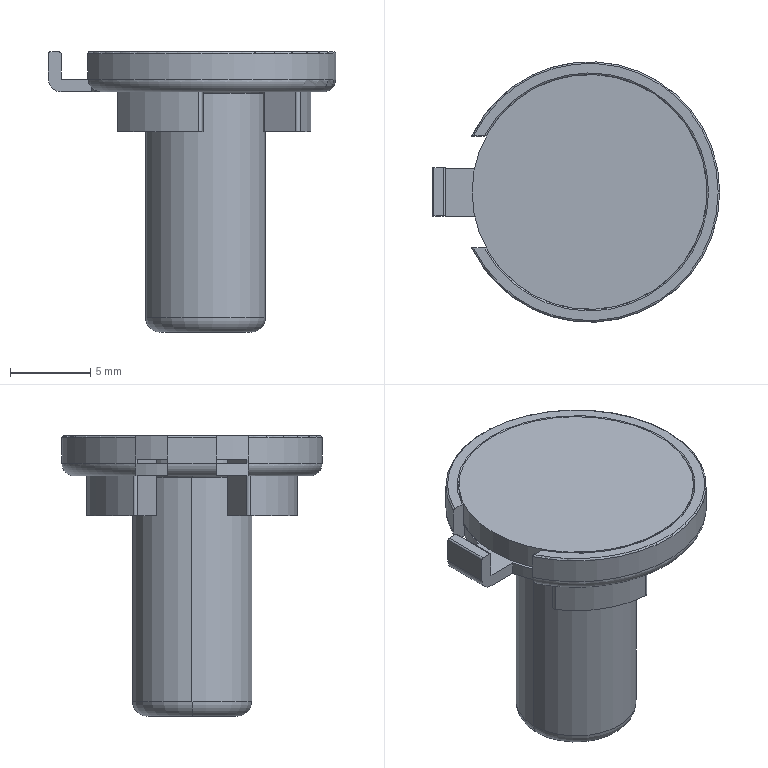NC program | NX | posted with a generic post | part box 17.958 x 16.273 x 17.5 mm
Lines 4450 to 5539 of 11029:
(ZLEVEL_PROFILE_COPY_COPY_2_COPY_1_COPY , TOOL : D1)
N8886 T12 M6
N8888 G54
N8890 G17 G0 G90 X-0.541 Y-4.574 S8005 M3
N8892 G43 Z30. H12
N8894 Z-0.08
N8896 G94 G1 X-0.394 Y-4.482 F850.
N8898 X-0.36 Y-4.465
N8900 X-0.342 Y-4.431
N8902 X-0.347 Y-4.394
N8904 X-0.353 Y-4.21
N8906 G2 X0.289 Y-3.488 R0.7
N8908 G3 X2.876 Y-1.994 R3.5
N8910 G2 X3.823 Y-1.799 R0.7
N8912 G1 X3.978 Y-1.896
N8914 X4.008 Y-1.919
N8916 X4.047 Y-1.92
N8918 X4.078 Y-1.9
N8920 X4.231 Y-1.819
N8922 G0 Z30.
N8924 Y1.819
N8926 Z-0.08
N8928 G1 X4.078 Y1.9
N8930 X4.047 Y1.92
N8932 X4.008 Y1.919
N8934 X3.978 Y1.896
N8936 X3.823 Y1.799
N8938 G2 X2.876 Y1.994 R0.7
N8940 G3 X0.289 Y3.488 R3.5
N8942 G2 X-0.353 Y4.21 R0.7
N8944 G1 X-0.347 Y4.394
N8946 X-0.342 Y4.431
N8948 X-0.36 Y4.465
N8950 X-0.394 Y4.482
N8952 X-0.541 Y4.574
N8954 G0 Z30.
N8956 X-3.69 Y2.755
N8958 Z-0.08
N8960 G1 X-3.684 Y2.582
N8962 X-3.687 Y2.544
N8964 X-3.666 Y2.512
N8966 X-3.631 Y2.497
N8968 X-3.469 Y2.411
N8970 G2 X-3.165 Y1.494 R0.7
N8972 G3 X-3.165 Y-1.494 R3.5
N8974 G2 X-3.469 Y-2.411 R0.7
N8976 G1 X-3.631 Y-2.497
N8978 X-3.666 Y-2.512
N8980 X-3.687 Y-2.544
N8982 X-3.684 Y-2.582
N8984 X-3.69 Y-2.755
N8986 G0 Z30.
N8988 X-2.316 Y-2.821
N8990 Z-0.08
N8992 G1 X-2.281 Y-2.656
N8994 X-2.27 Y-2.62
N8996 X-2.281 Y-2.584
N8998 X-2.312 Y-2.561
N9000 G2 X-2.312 Y2.561 R3.45
N9002 G1 X-2.281 Y2.584
N9004 X-2.27 Y2.62
N9006 X-2.281 Y2.656
N9008 X-2.316 Y2.821
N9010 G0 Z30.
N9012 Y-2.821
N9014 Z-0.159
N9016 G1 X-2.281 Y-2.656
N9018 X-2.27 Y-2.62
N9020 X-2.281 Y-2.584
N9022 X-2.312 Y-2.561
N9024 G2 X-2.312 Y2.561 R3.45
N9026 G1 X-2.281 Y2.584
N9028 X-2.27 Y2.62
N9030 X-2.281 Y2.656
N9032 X-2.316 Y2.821
N9034 G0 Z30.
N9036 X-3.69 Y2.755
N9038 Z-0.159
N9040 G1 X-3.684 Y2.582
N9042 X-3.687 Y2.544
N9044 X-3.666 Y2.512
N9046 X-3.631 Y2.497
N9048 X-3.469 Y2.411
N9050 G2 X-3.165 Y1.494 R0.7
N9052 G3 X-3.165 Y-1.494 R3.5
N9054 G2 X-3.469 Y-2.411 R0.7
N9056 G1 X-3.631 Y-2.497
N9058 X-3.666 Y-2.512
N9060 X-3.687 Y-2.544
N9062 X-3.684 Y-2.582
N9064 X-3.69 Y-2.755
N9066 G0 Z30.
N9068 Y2.755
N9070 Z-0.239
N9072 G1 X-3.684 Y2.582
N9074 X-3.687 Y2.544
N9076 X-3.666 Y2.512
N9078 X-3.631 Y2.497
N9080 X-3.469 Y2.411
N9082 G2 X-3.165 Y1.494 R0.7
N9084 G3 X-3.165 Y-1.494 R3.5
N9086 G2 X-3.469 Y-2.411 R0.7
N9088 G1 X-3.631 Y-2.497
N9090 X-3.666 Y-2.512
N9092 X-3.687 Y-2.544
N9094 X-3.684 Y-2.582
N9096 X-3.69 Y-2.755
N9098 G0 Z30.
N9100 X-2.316 Y-2.821
N9102 Z-0.239
N9104 G1 X-2.281 Y-2.656
N9106 X-2.27 Y-2.62
N9108 X-2.281 Y-2.584
N9110 X-2.312 Y-2.561
N9112 G2 X-2.312 Y2.561 R3.45
N9114 G1 X-2.281 Y2.584
N9116 X-2.27 Y2.62
N9118 X-2.281 Y2.656
N9120 X-2.316 Y2.821
N9122 G0 Z30.
N9124 Y-2.821
N9126 Z-0.318
N9128 G1 X-2.281 Y-2.656
N9130 X-2.27 Y-2.62
N9132 X-2.281 Y-2.584
N9134 X-2.312 Y-2.561
N9136 G2 X-2.312 Y2.561 R3.45
N9138 G1 X-2.281 Y2.584
N9140 X-2.27 Y2.62
N9142 X-2.281 Y2.656
N9144 X-2.316 Y2.821
N9146 G0 Z30.
N9148 X-3.69 Y2.755
N9150 Z-0.318
N9152 G1 X-3.684 Y2.582
N9154 X-3.687 Y2.544
N9156 X-3.666 Y2.512
N9158 X-3.631 Y2.497
N9160 X-3.469 Y2.411
N9162 G2 X-3.165 Y1.494 R0.7
N9164 G3 X-3.165 Y-1.494 R3.5
N9166 G2 X-3.469 Y-2.411 R0.7
N9168 G1 X-3.631 Y-2.497
N9170 X-3.666 Y-2.512
N9172 X-3.687 Y-2.544
N9174 X-3.684 Y-2.582
N9176 X-3.69 Y-2.755
N9178 G0 Z30.
N9180 Y2.755
N9182 Z-0.398
N9184 G1 X-3.684 Y2.582
N9186 X-3.687 Y2.544
N9188 X-3.666 Y2.512
N9190 X-3.631 Y2.497
N9192 X-3.469 Y2.411
N9194 G2 X-3.165 Y1.494 R0.7
N9196 G3 X-3.165 Y-1.494 R3.5
N9198 G2 X-3.469 Y-2.411 R0.7
N9200 G1 X-3.631 Y-2.497
N9202 X-3.666 Y-2.512
N9204 X-3.687 Y-2.544
N9206 X-3.684 Y-2.582
N9208 X-3.69 Y-2.755
N9210 G0 Z30.
N9212 X-2.316 Y-2.821
N9214 Z-0.398
N9216 G1 X-2.281 Y-2.656
N9218 X-2.27 Y-2.62
N9220 X-2.281 Y-2.584
N9222 X-2.312 Y-2.561
N9224 G2 X-2.312 Y2.561 R3.45
N9226 G1 X-2.281 Y2.584
N9228 X-2.27 Y2.62
N9230 X-2.281 Y2.656
N9232 X-2.316 Y2.821
N9234 G0 Z30.
N9236 Y-2.821
N9238 Z-0.477
N9240 G1 X-2.281 Y-2.656
N9242 X-2.27 Y-2.62
N9244 X-2.281 Y-2.584
N9246 X-2.312 Y-2.561
N9248 G2 X-2.312 Y2.561 R3.45
N9250 G1 X-2.281 Y2.584
N9252 X-2.27 Y2.62
N9254 X-2.281 Y2.656
N9256 X-2.316 Y2.821
N9258 G0 Z30.
N9260 X-3.69 Y2.755
N9262 Z-0.477
N9264 G1 X-3.684 Y2.582
N9266 X-3.687 Y2.544
N9268 X-3.666 Y2.512
N9270 X-3.631 Y2.497
N9272 X-3.469 Y2.411
N9274 G2 X-3.165 Y1.494 R0.7
N9276 G3 X-3.165 Y-1.494 R3.5
N9278 G2 X-3.469 Y-2.411 R0.7
N9280 G1 X-3.631 Y-2.497
N9282 X-3.666 Y-2.512
N9284 X-3.687 Y-2.544
N9286 X-3.684 Y-2.582
N9288 X-3.69 Y-2.755
N9290 G0 Z30.
N9292 Y2.755
N9294 Z-0.557
N9296 G1 X-3.684 Y2.582
N9298 X-3.687 Y2.544
N9300 X-3.666 Y2.512
N9302 X-3.631 Y2.497
N9304 X-3.469 Y2.411
N9306 G2 X-3.165 Y1.494 R0.7
N9308 G3 X-3.165 Y-1.494 R3.5
N9310 G2 X-3.469 Y-2.411 R0.7
N9312 G1 X-3.631 Y-2.497
N9314 X-3.666 Y-2.512
N9316 X-3.687 Y-2.544
N9318 X-3.684 Y-2.582
N9320 X-3.69 Y-2.755
N9322 G0 Z30.
N9324 X-2.316 Y-2.821
N9326 Z-0.557
N9328 G1 X-2.281 Y-2.656
N9330 X-2.27 Y-2.62
N9332 X-2.281 Y-2.584
N9334 X-2.312 Y-2.561
N9336 G2 X-2.312 Y2.561 R3.45
N9338 G1 X-2.281 Y2.584
N9340 X-2.27 Y2.62
N9342 X-2.281 Y2.656
N9344 X-2.316 Y2.821
N9346 G0 Z30.
N9348 Y-2.821
N9350 Z-0.636
N9352 G1 X-2.281 Y-2.656
N9354 X-2.27 Y-2.62
N9356 X-2.281 Y-2.584
N9358 X-2.312 Y-2.561
N9360 G2 X-2.312 Y2.561 R3.45
N9362 G1 X-2.281 Y2.584
N9364 X-2.27 Y2.62
N9366 X-2.281 Y2.656
N9368 X-2.316 Y2.821
N9370 G0 Z30.
N9372 X-3.69 Y2.755
N9374 Z-0.636
N9376 G1 X-3.684 Y2.582
N9378 X-3.687 Y2.544
N9380 X-3.666 Y2.512
N9382 X-3.631 Y2.497
N9384 X-3.469 Y2.411
N9386 G2 X-3.165 Y1.494 R0.7
N9388 G3 X-3.165 Y-1.494 R3.5
N9390 G2 X-3.469 Y-2.411 R0.7
N9392 G1 X-3.631 Y-2.497
N9394 X-3.666 Y-2.512
N9396 X-3.687 Y-2.544
N9398 X-3.684 Y-2.582
N9400 X-3.69 Y-2.755
N9402 G0 Z30.
N9404 Y2.755
N9406 Z-0.716
N9408 G1 X-3.684 Y2.582
N9410 X-3.687 Y2.544
N9412 X-3.666 Y2.512
N9414 X-3.631 Y2.497
N9416 X-3.469 Y2.411
N9418 G2 X-3.165 Y1.494 R0.7
N9420 G3 X-3.165 Y-1.494 R3.5
N9422 G2 X-3.469 Y-2.411 R0.7
N9424 G1 X-3.631 Y-2.497
N9426 X-3.666 Y-2.512
N9428 X-3.687 Y-2.544
N9430 X-3.684 Y-2.582
N9432 X-3.69 Y-2.755
N9434 G0 Z30.
N9436 X-2.316 Y-2.821
N9438 Z-0.716
N9440 G1 X-2.281 Y-2.656
N9442 X-2.27 Y-2.62
N9444 X-2.281 Y-2.584
N9446 X-2.312 Y-2.561
N9448 G2 X-2.312 Y2.561 R3.45
N9450 G1 X-2.281 Y2.584
N9452 X-2.27 Y2.62
N9454 X-2.281 Y2.656
N9456 X-2.316 Y2.821
N9458 G0 Z30.
N9460 Y-2.821
N9462 Z-0.795
N9464 G1 X-2.281 Y-2.656
N9466 X-2.27 Y-2.62
N9468 X-2.281 Y-2.584
N9470 X-2.312 Y-2.561
N9472 G2 X-2.312 Y2.561 R3.45
N9474 G1 X-2.281 Y2.584
N9476 X-2.27 Y2.62
N9478 X-2.281 Y2.656
N9480 X-2.316 Y2.821
N9482 G0 Z30.
N9484 X-3.69 Y2.755
N9486 Z-0.795
N9488 G1 X-3.684 Y2.582
N9490 X-3.687 Y2.544
N9492 X-3.666 Y2.512
N9494 X-3.631 Y2.497
N9496 X-3.469 Y2.411
N9498 G2 X-3.165 Y1.494 R0.7
N9500 G3 X-3.165 Y-1.494 R3.5
N9502 G2 X-3.469 Y-2.411 R0.7
N9504 G1 X-3.631 Y-2.497
N9506 X-3.666 Y-2.512
N9508 X-3.687 Y-2.544
N9510 X-3.684 Y-2.582
N9512 X-3.69 Y-2.755
N9514 G0 Z30.
N9516 Y2.755
N9518 Z-0.875
N9520 G1 X-3.684 Y2.582
N9522 X-3.687 Y2.544
N9524 X-3.666 Y2.512
N9526 X-3.631 Y2.497
N9528 X-3.469 Y2.411
N9530 G2 X-3.165 Y1.494 R0.7
N9532 G3 X-3.165 Y-1.494 R3.5
N9534 G2 X-3.469 Y-2.411 R0.7
N9536 G1 X-3.631 Y-2.497
N9538 X-3.666 Y-2.512
N9540 X-3.687 Y-2.544
N9542 X-3.684 Y-2.582
N9544 X-3.69 Y-2.755
N9546 G0 Z30.
N9548 X-2.316 Y-2.821
N9550 Z-0.875
N9552 G1 X-2.281 Y-2.656
N9554 X-2.27 Y-2.62
N9556 X-2.281 Y-2.584
N9558 X-2.312 Y-2.561
N9560 G2 X-2.312 Y2.561 R3.45
N9562 G1 X-2.281 Y2.584
N9564 X-2.27 Y2.62
N9566 X-2.281 Y2.656
N9568 X-2.316 Y2.821
N9570 G0 Z30.
N9572 Y-2.821
N9574 Z-0.955
N9576 G1 X-2.281 Y-2.656
N9578 X-2.27 Y-2.62
N9580 X-2.281 Y-2.584
N9582 X-2.312 Y-2.561
N9584 G2 X-2.312 Y2.561 R3.45
N9586 G1 X-2.281 Y2.584
N9588 X-2.27 Y2.62
N9590 X-2.281 Y2.656
N9592 X-2.316 Y2.821
N9594 G0 Z30.
N9596 X-3.69 Y2.755
N9598 Z-0.955
N9600 G1 X-3.684 Y2.582
N9602 X-3.687 Y2.544
N9604 X-3.666 Y2.512
N9606 X-3.631 Y2.497
N9608 X-3.469 Y2.411
N9610 G2 X-3.165 Y1.494 R0.7
N9612 G3 X-3.165 Y-1.494 R3.5
N9614 G2 X-3.469 Y-2.411 R0.7
N9616 G1 X-3.631 Y-2.497
N9618 X-3.666 Y-2.512
N9620 X-3.687 Y-2.544
N9622 X-3.684 Y-2.582
N9624 X-3.69 Y-2.755
N9626 G0 Z30.
N9628 Y2.755
N9630 Z-1.034
N9632 G1 X-3.684 Y2.582
N9634 X-3.687 Y2.544
N9636 X-3.666 Y2.512
N9638 X-3.631 Y2.497
N9640 X-3.469 Y2.411
N9642 G2 X-3.165 Y1.494 R0.7
N9644 G3 X-3.165 Y-1.494 R3.5
N9646 G2 X-3.469 Y-2.411 R0.7
N9648 G1 X-3.631 Y-2.497
N9650 X-3.666 Y-2.512
N9652 X-3.687 Y-2.544
N9654 X-3.684 Y-2.582
N9656 X-3.69 Y-2.755
N9658 G0 Z30.
N9660 X-2.316 Y-2.821
N9662 Z-1.034
N9664 G1 X-2.281 Y-2.656
N9666 X-2.27 Y-2.62
N9668 X-2.281 Y-2.584
N9670 X-2.312 Y-2.561
N9672 G2 X-2.312 Y2.561 R3.45
N9674 G1 X-2.281 Y2.584
N9676 X-2.27 Y2.62
N9678 X-2.281 Y2.656
N9680 X-2.316 Y2.821
N9682 G0 Z30.
N9684 Y-2.821
N9686 Z-1.114
N9688 G1 X-2.281 Y-2.656
N9690 X-2.27 Y-2.62
N9692 X-2.281 Y-2.584
N9694 X-2.312 Y-2.561
N9696 G2 X-2.312 Y2.561 R3.45
N9698 G1 X-2.281 Y2.584
N9700 X-2.27 Y2.62
N9702 X-2.281 Y2.656
N9704 X-2.316 Y2.821
N9706 G0 Z30.
N9708 X-3.69 Y2.755
N9710 Z-1.114
N9712 G1 X-3.684 Y2.582
N9714 X-3.687 Y2.544
N9716 X-3.666 Y2.512
N9718 X-3.631 Y2.497
N9720 X-3.469 Y2.411
N9722 G2 X-3.165 Y1.494 R0.7
N9724 G3 X-3.165 Y-1.494 R3.5
N9726 G2 X-3.469 Y-2.411 R0.7
N9728 G1 X-3.631 Y-2.497
N9730 X-3.666 Y-2.512
N9732 X-3.687 Y-2.544
N9734 X-3.684 Y-2.582
N9736 X-3.69 Y-2.755
N9738 G0 Z30.
N9740 Y2.755
N9742 Z-1.193
N9744 G1 X-3.684 Y2.582
N9746 X-3.687 Y2.544
N9748 X-3.666 Y2.512
N9750 X-3.631 Y2.497
N9752 X-3.469 Y2.411
N9754 G2 X-3.165 Y1.494 R0.7
N9756 G3 X-3.165 Y-1.494 R3.5
N9758 G2 X-3.469 Y-2.411 R0.7
N9760 G1 X-3.631 Y-2.497
N9762 X-3.666 Y-2.512
N9764 X-3.687 Y-2.544
N9766 X-3.684 Y-2.582
N9768 X-3.69 Y-2.755
N9770 G0 Z30.
N9772 X-2.316 Y-2.821
N9774 Z-1.193
N9776 G1 X-2.281 Y-2.656
N9778 X-2.27 Y-2.62
N9780 X-2.281 Y-2.584
N9782 X-2.312 Y-2.561
N9784 G2 X-2.312 Y2.561 R3.45
N9786 G1 X-2.281 Y2.584
N9788 X-2.27 Y2.62
N9790 X-2.281 Y2.656
N9792 X-2.316 Y2.821
N9794 G0 Z30.
N9796 Y-2.821
N9798 Z-1.273
N9800 G1 X-2.281 Y-2.656
N9802 X-2.27 Y-2.62
N9804 X-2.281 Y-2.584
N9806 X-2.312 Y-2.561
N9808 G2 X-2.312 Y2.561 R3.45
N9810 G1 X-2.281 Y2.584
N9812 X-2.27 Y2.62
N9814 X-2.281 Y2.656
N9816 X-2.316 Y2.821
N9818 G0 Z30.
N9820 X-3.69 Y2.755
N9822 Z-1.273
N9824 G1 X-3.684 Y2.582
N9826 X-3.687 Y2.544
N9828 X-3.666 Y2.512
N9830 X-3.631 Y2.497
N9832 X-3.469 Y2.411
N9834 G2 X-3.165 Y1.494 R0.7
N9836 G3 X-3.165 Y-1.494 R3.5
N9838 G2 X-3.469 Y-2.411 R0.7
N9840 G1 X-3.631 Y-2.497
N9842 X-3.666 Y-2.512
N9844 X-3.687 Y-2.544
N9846 X-3.684 Y-2.582
N9848 X-3.69 Y-2.755
N9850 G0 Z30.
N9852 Y2.755
N9854 Z-1.352
N9856 G1 X-3.684 Y2.582
N9858 X-3.687 Y2.544
N9860 X-3.666 Y2.512
N9862 X-3.631 Y2.497
N9864 X-3.469 Y2.411
N9866 G2 X-3.165 Y1.494 R0.7
N9868 G3 X-3.165 Y-1.494 R3.5
N9870 G2 X-3.469 Y-2.411 R0.7
N9872 G1 X-3.631 Y-2.497
N9874 X-3.666 Y-2.512
N9876 X-3.687 Y-2.544
N9878 X-3.684 Y-2.582
N9880 X-3.69 Y-2.755
N9882 G0 Z30.
N9884 X-2.316 Y-2.821
N9886 Z-1.352
N9888 G1 X-2.281 Y-2.656
N9890 X-2.27 Y-2.62
N9892 X-2.281 Y-2.584
N9894 X-2.312 Y-2.561
N9896 G2 X-2.312 Y2.561 R3.45
N9898 G1 X-2.281 Y2.584
N9900 X-2.27 Y2.62
N9902 X-2.281 Y2.656
N9904 X-2.316 Y2.821
N9906 G0 Z30.
N9908 Y-2.821
N9910 Z-1.432
N9912 G1 X-2.281 Y-2.656
N9914 X-2.27 Y-2.62
N9916 X-2.281 Y-2.584
N9918 X-2.312 Y-2.561
N9920 G2 X-2.312 Y2.561 R3.45
N9922 G1 X-2.281 Y2.584
N9924 X-2.27 Y2.62
N9926 X-2.281 Y2.656
N9928 X-2.316 Y2.821
N9930 G0 Z30.
N9932 X-3.69 Y2.755
N9934 Z-1.432
N9936 G1 X-3.684 Y2.582
N9938 X-3.687 Y2.544
N9940 X-3.666 Y2.512
N9942 X-3.631 Y2.497
N9944 X-3.469 Y2.411
N9946 G2 X-3.165 Y1.494 R0.7
N9948 G3 X-3.165 Y-1.494 R3.5
N9950 G2 X-3.469 Y-2.411 R0.7
N9952 G1 X-3.631 Y-2.497
N9954 X-3.666 Y-2.512
N9956 X-3.687 Y-2.544
N9958 X-3.684 Y-2.582
N9960 X-3.69 Y-2.755
N9962 G0 Z30.
N9964 Y2.755
N9966 Z-1.511
N9968 G1 X-3.684 Y2.582
N9970 X-3.687 Y2.544
N9972 X-3.666 Y2.512
N9974 X-3.631 Y2.497
N9976 X-3.469 Y2.411
N9978 G2 X-3.165 Y1.494 R0.7
N9980 G3 X-3.165 Y-1.494 R3.5
N9982 G2 X-3.469 Y-2.411 R0.7
N9984 G1 X-3.631 Y-2.497
N9986 X-3.666 Y-2.512
N9988 X-3.687 Y-2.544
N9990 X-3.684 Y-2.582
N9992 X-3.69 Y-2.755
N9994 G0 Z30.
N9996 X-2.316 Y-2.821
N9998 Z-1.511
N10000 G1 X-2.281 Y-2.656
N10002 X-2.27 Y-2.62
N10004 X-2.281 Y-2.584
N10006 X-2.312 Y-2.561
N10008 G2 X-2.312 Y2.561 R3.45
N10010 G1 X-2.281 Y2.584
N10012 X-2.27 Y2.62
N10014 X-2.281 Y2.656
N10016 X-2.316 Y2.821
N10018 G0 Z30.
N10020 Y-2.821
N10022 Z-1.591
N10024 G1 X-2.281 Y-2.656
N10026 X-2.27 Y-2.62
N10028 X-2.281 Y-2.584
N10030 X-2.312 Y-2.561
N10032 G2 X-2.312 Y2.561 R3.45
N10034 G1 X-2.281 Y2.584
N10036 X-2.27 Y2.62
N10038 X-2.281 Y2.656
N10040 X-2.316 Y2.821
N10042 G0 Z30.
N10044 X-3.69 Y2.755
N10046 Z-1.591
N10048 G1 X-3.684 Y2.582
N10050 X-3.687 Y2.544
N10052 X-3.666 Y2.512
N10054 X-3.631 Y2.497
N10056 X-3.469 Y2.411
N10058 G2 X-3.165 Y1.494 R0.7
N10060 G3 X-3.165 Y-1.494 R3.5
N10062 G2 X-3.469 Y-2.411 R0.7
N10064 G1 X-3.631 Y-2.497
N10066 X-3.666 Y-2.512
N10068 X-3.687 Y-2.544
N10070 X-3.684 Y-2.582
N10072 X-3.69 Y-2.755
N10074 G0 Z30.
N10076 Y2.755
N10078 Z-1.67
N10080 G1 X-3.684 Y2.582
N10082 X-3.687 Y2.544
N10084 X-3.666 Y2.512
N10086 X-3.631 Y2.497
N10088 X-3.469 Y2.411
N10090 G2 X-3.165 Y1.494 R0.7
N10092 G3 X-3.165 Y-1.494 R3.5
N10094 G2 X-3.469 Y-2.411 R0.7
N10096 G1 X-3.631 Y-2.497
N10098 X-3.666 Y-2.512
N10100 X-3.687 Y-2.544
N10102 X-3.684 Y-2.582
N10104 X-3.69 Y-2.755
N10106 G0 Z30.
N10108 X-2.316 Y-2.821
N10110 Z-1.67
N10112 G1 X-2.281 Y-2.656
N10114 X-2.27 Y-2.62
N10116 X-2.281 Y-2.584
N10118 X-2.312 Y-2.561
N10120 G2 X-2.312 Y2.561 R3.45
N10122 G1 X-2.281 Y2.584
N10124 X-2.27 Y2.62
N10126 X-2.281 Y2.656
N10128 X-2.316 Y2.821
N10130 G0 Z30.
N10132 Y-2.821
N10134 Z-1.75
N10136 G1 X-2.281 Y-2.656
N10138 X-2.27 Y-2.62
N10140 X-2.281 Y-2.584
N10142 X-2.312 Y-2.561
N10144 G2 X-2.312 Y2.561 R3.45
N10146 G1 X-2.281 Y2.584
N10148 X-2.27 Y2.62
N10150 X-2.281 Y2.656
N10152 X-2.316 Y2.821
N10154 G0 Z30.
N10156 X-3.69 Y2.755
N10158 Z-1.75
N10160 G1 X-3.684 Y2.582
N10162 X-3.687 Y2.544
N10164 X-3.666 Y2.512
N10166 X-3.631 Y2.497
N10168 X-3.469 Y2.411
N10170 G2 X-3.165 Y1.494 R0.7
N10172 G3 X-3.165 Y-1.494 R3.5
N10174 G2 X-3.469 Y-2.411 R0.7
N10176 G1 X-3.631 Y-2.497
N10178 X-3.666 Y-2.512
N10180 X-3.687 Y-2.544
N10182 X-3.684 Y-2.582
N10184 X-3.69 Y-2.755
N10186 G0 Z30.
N10188 Y2.755
N10190 Z-1.83
N10192 G1 X-3.684 Y2.582
N10194 X-3.687 Y2.544
N10196 X-3.666 Y2.512
N10198 X-3.631 Y2.497
N10200 X-3.469 Y2.411
N10202 G2 X-3.165 Y1.494 R0.7
N10204 G3 X-3.165 Y-1.494 R3.5
N10206 G2 X-3.469 Y-2.411 R0.7
N10208 G1 X-3.631 Y-2.497
N10210 X-3.666 Y-2.512
N10212 X-3.687 Y-2.544
N10214 X-3.684 Y-2.582
N10216 X-3.69 Y-2.755
N10218 G0 Z30.
N10220 X-2.316 Y-2.821
N10222 Z-1.83
N10224 G1 X-2.281 Y-2.656
N10226 X-2.27 Y-2.62
N10228 X-2.281 Y-2.584
N10230 X-2.312 Y-2.561
N10232 G2 X-2.312 Y2.561 R3.45
N10234 G1 X-2.281 Y2.584
N10236 X-2.27 Y2.62
N10238 X-2.281 Y2.656
N10240 X-2.316 Y2.821
N10242 G0 Z30.
N10244 Y-2.821
N10246 Z-1.909
N10248 G1 X-2.281 Y-2.656
N10250 X-2.27 Y-2.62
N10252 X-2.281 Y-2.584
N10254 X-2.312 Y-2.561
N10256 G2 X-2.312 Y2.561 R3.45
N10258 G1 X-2.281 Y2.584
N10260 X-2.27 Y2.62
N10262 X-2.281 Y2.656
N10264 X-2.316 Y2.821
N10266 G0 Z30.
N10268 X-3.69 Y2.755
N10270 Z-1.909
N10272 G1 X-3.684 Y2.582
N10274 X-3.687 Y2.544
N10276 X-3.666 Y2.512
N10278 X-3.631 Y2.497
N10280 X-3.469 Y2.411
N10282 G2 X-3.165 Y1.494 R0.7
N10284 G3 X-3.165 Y-1.494 R3.5
N10286 G2 X-3.469 Y-2.411 R0.7
N10288 G1 X-3.631 Y-2.497
N10290 X-3.666 Y-2.512
N10292 X-3.687 Y-2.544
N10294 X-3.684 Y-2.582
N10296 X-3.69 Y-2.755
N10298 G0 Z30.
N10300 Y2.755
N10302 Z-1.989
N10304 G1 X-3.684 Y2.582
N10306 X-3.687 Y2.544
N10308 X-3.666 Y2.512
N10310 X-3.631 Y2.497
N10312 X-3.469 Y2.411
N10314 G2 X-3.165 Y1.494 R0.7
N10316 G3 X-3.165 Y-1.494 R3.5
N10318 G2 X-3.469 Y-2.411 R0.7
N10320 G1 X-3.631 Y-2.497
N10322 X-3.666 Y-2.512
N10324 X-3.687 Y-2.544
N10326 X-3.684 Y-2.582
N10328 X-3.69 Y-2.755
N10330 G0 Z30.
N10332 X-2.316 Y-2.821
N10334 Z-1.989
N10336 G1 X-2.281 Y-2.656
N10338 X-2.27 Y-2.62
N10340 X-2.281 Y-2.584
N10342 X-2.312 Y-2.561
N10344 G2 X-2.312 Y2.561 R3.45
N10346 G1 X-2.281 Y2.584
N10348 X-2.27 Y2.62
N10350 X-2.281 Y2.656
N10352 X-2.316 Y2.821
N10354 G0 Z30.
N10356 Y-2.821
N10358 Z-2.068
N10360 G1 X-2.281 Y-2.656
N10362 X-2.27 Y-2.62
N10364 X-2.281 Y-2.584
N10366 X-2.312 Y-2.561
N10368 G2 X-2.312 Y2.561 R3.45
N10370 G1 X-2.281 Y2.584
N10372 X-2.27 Y2.62
N10374 X-2.281 Y2.656
N10376 X-2.316 Y2.821
N10378 G0 Z30.
N10380 X-3.69 Y2.755
N10382 Z-2.068
N10384 G1 X-3.684 Y2.582
N10386 X-3.687 Y2.544
N10388 X-3.666 Y2.512
N10390 X-3.631 Y2.497
N10392 X-3.469 Y2.411
N10394 G2 X-3.165 Y1.494 R0.7
N10396 G3 X-3.165 Y-1.494 R3.5
N10398 G2 X-3.469 Y-2.411 R0.7
N10400 G1 X-3.631 Y-2.497
N10402 X-3.666 Y-2.512
N10404 X-3.687 Y-2.544
N10406 X-3.684 Y-2.582
N10408 X-3.69 Y-2.755
N10410 G0 Z30.
N10412 Y2.755
N10414 Z-2.148
N10416 G1 X-3.684 Y2.582
N10418 X-3.687 Y2.544
N10420 X-3.666 Y2.512
N10422 X-3.631 Y2.497
N10424 X-3.469 Y2.411
N10426 G2 X-3.165 Y1.494 R0.7
N10428 G3 X-3.165 Y-1.494 R3.5
N10430 G2 X-3.469 Y-2.411 R0.7
N10432 G1 X-3.631 Y-2.497
N10434 X-3.666 Y-2.512
N10436 X-3.687 Y-2.544
N10438 X-3.684 Y-2.582
N10440 X-3.69 Y-2.755
N10442 G0 Z30.
N10444 X-2.316 Y-2.821
N10446 Z-2.148
N10448 G1 X-2.281 Y-2.656
N10450 X-2.27 Y-2.62
N10452 X-2.281 Y-2.584
N10454 X-2.312 Y-2.561
N10456 G2 X-2.312 Y2.561 R3.45
N10458 G1 X-2.281 Y2.584
N10460 X-2.27 Y2.62
N10462 X-2.281 Y2.656
N10464 X-2.316 Y2.821
N10466 G0 Z30.
N10468 Y-2.821
N10470 Z-2.227
N10472 G1 X-2.281 Y-2.656
N10474 X-2.27 Y-2.62
N10476 X-2.281 Y-2.584
N10478 X-2.312 Y-2.561
N10480 G2 X-2.312 Y2.561 R3.45
N10482 G1 X-2.281 Y2.584
N10484 X-2.27 Y2.62
N10486 X-2.281 Y2.656
N10488 X-2.316 Y2.821
N10490 G0 Z30.
N10492 X-3.69 Y2.755
N10494 Z-2.227
N10496 G1 X-3.684 Y2.582
N10498 X-3.687 Y2.544
N10500 X-3.666 Y2.512
N10502 X-3.631 Y2.497
N10504 X-3.469 Y2.411
N10506 G2 X-3.165 Y1.494 R0.7
N10508 G3 X-3.165 Y-1.494 R3.5
N10510 G2 X-3.469 Y-2.411 R0.7
N10512 G1 X-3.631 Y-2.497
N10514 X-3.666 Y-2.512
N10516 X-3.687 Y-2.544
N10518 X-3.684 Y-2.582
N10520 X-3.69 Y-2.755
N10522 G0 Z30.
N10524 Y2.755
N10526 Z-2.307
N10528 G1 X-3.684 Y2.582
N10530 X-3.687 Y2.544
N10532 X-3.666 Y2.512
N10534 X-3.631 Y2.497
N10536 X-3.469 Y2.411
N10538 G2 X-3.165 Y1.494 R0.7
N10540 G3 X-3.165 Y-1.494 R3.5
N10542 G2 X-3.469 Y-2.411 R0.7
N10544 G1 X-3.631 Y-2.497
N10546 X-3.666 Y-2.512
N10548 X-3.687 Y-2.544
N10550 X-3.684 Y-2.582
N10552 X-3.69 Y-2.755
N10554 G0 Z30.
N10556 X-2.316 Y-2.821
N10558 Z-2.307
N10560 G1 X-2.281 Y-2.656
N10562 X-2.27 Y-2.62
N10564 X-2.281 Y-2.584
N10566 X-2.312 Y-2.561
N10568 G2 X-2.312 Y2.561 R3.45
N10570 G1 X-2.281 Y2.584
N10572 X-2.27 Y2.62
N10574 X-2.281 Y2.656
N10576 X-2.316 Y2.821
N10578 G0 Z30.
N10580 Y-2.821
N10582 Z-2.386
N10584 G1 X-2.281 Y-2.656
N10586 X-2.27 Y-2.62
N10588 X-2.281 Y-2.584
N10590 X-2.312 Y-2.561
N10592 G2 X-2.312 Y2.561 R3.45
N10594 G1 X-2.281 Y2.584
N10596 X-2.27 Y2.62
N10598 X-2.281 Y2.656
N10600 X-2.316 Y2.821
N10602 G0 Z30.
N10604 X-3.69 Y2.755
N10606 Z-2.386
N10608 G1 X-3.684 Y2.582
N10610 X-3.687 Y2.544
N10612 X-3.666 Y2.512
N10614 X-3.631 Y2.497
N10616 X-3.469 Y2.411
N10618 G2 X-3.165 Y1.494 R0.7
N10620 G3 X-3.165 Y-1.494 R3.5
N10622 G2 X-3.469 Y-2.411 R0.7
N10624 G1 X-3.631 Y-2.497
N10626 X-3.666 Y-2.512
N10628 X-3.687 Y-2.544
N10630 X-3.684 Y-2.582
N10632 X-3.69 Y-2.755
N10634 G0 Z30.
N10636 Y2.755
N10638 Z-2.466
N10640 G1 X-3.684 Y2.582
N10642 X-3.687 Y2.544
N10644 X-3.666 Y2.512
N10646 X-3.631 Y2.497
N10648 X-3.469 Y2.411
N10650 G2 X-3.165 Y1.494 R0.7
N10652 G3 X-3.165 Y-1.494 R3.5
N10654 G2 X-3.469 Y-2.411 R0.7
N10656 G1 X-3.631 Y-2.497
N10658 X-3.666 Y-2.512
N10660 X-3.687 Y-2.544
N10662 X-3.684 Y-2.582
N10664 X-3.69 Y-2.755
N10666 G0 Z30.
N10668 X-2.316 Y-2.821
N10670 Z-2.466
N10672 G1 X-2.281 Y-2.656
N10674 X-2.27 Y-2.62
N10676 X-2.281 Y-2.584
N10678 X-2.312 Y-2.561
N10680 G2 X-2.312 Y2.561 R3.45
N10682 G1 X-2.281 Y2.584
N10684 X-2.27 Y2.62
N10686 X-2.281 Y2.656
N10688 X-2.316 Y2.821
N10690 G0 Z30.
N10692 Y-2.821
N10694 Z-2.545
N10696 G1 X-2.281 Y-2.656
N10698 X-2.27 Y-2.62
N10700 X-2.281 Y-2.584
N10702 X-2.312 Y-2.561
N10704 G2 X-2.312 Y2.561 R3.45
N10706 G1 X-2.281 Y2.584
N10708 X-2.27 Y2.62
N10710 X-2.281 Y2.656
N10712 X-2.316 Y2.821
N10714 G0 Z30.
N10716 X-3.69 Y2.755
N10718 Z-2.545
N10720 G1 X-3.684 Y2.582
N10722 X-3.687 Y2.544
N10724 X-3.666 Y2.512
N10726 X-3.631 Y2.497
N10728 X-3.469 Y2.411
N10730 G2 X-3.165 Y1.494 R0.7
N10732 G3 X-3.165 Y-1.494 R3.5
N10734 G2 X-3.469 Y-2.411 R0.7
N10736 G1 X-3.631 Y-2.497
N10738 X-3.666 Y-2.512
N10740 X-3.687 Y-2.544
N10742 X-3.684 Y-2.582
N10744 X-3.69 Y-2.755
N10746 G0 Z30.
N10748 Y2.755
N10750 Z-2.625
N10752 G1 X-3.684 Y2.582
N10754 X-3.687 Y2.544
N10756 X-3.666 Y2.512
N10758 X-3.631 Y2.497
N10760 X-3.469 Y2.411
N10762 G2 X-3.165 Y1.494 R0.7
N10764 G3 X-3.165 Y-1.494 R3.5
N10766 G2 X-3.469 Y-2.411 R0.7
N10768 G1 X-3.631 Y-2.497
N10770 X-3.666 Y-2.512
N10772 X-3.687 Y-2.544
N10774 X-3.684 Y-2.582
N10776 X-3.69 Y-2.755
N10778 G0 Z30.
N10780 X-2.316 Y-2.821
N10782 Z-2.625
N10784 G1 X-2.281 Y-2.656
N10786 X-2.27 Y-2.62
N10788 X-2.281 Y-2.584
N10790 X-2.312 Y-2.561
N10792 G2 X-2.312 Y2.561 R3.45
N10794 G1 X-2.281 Y2.584
N10796 X-2.27 Y2.62
N10798 X-2.281 Y2.656
N10800 X-2.316 Y2.821
N10802 G0 Z30.
N10804 Y-2.821
N10806 Z-2.705
N10808 G1 X-2.281 Y-2.656
N10810 X-2.27 Y-2.62
N10812 X-2.281 Y-2.584
N10814 X-2.312 Y-2.561
N10816 G2 X-2.312 Y2.561 R3.45
N10818 G1 X-2.281 Y2.584
N10820 X-2.27 Y2.62
N10822 X-2.281 Y2.656
N10824 X-2.316 Y2.821
N10826 G0 Z30.
N10828 X-3.69 Y2.755
N10830 Z-2.705
N10832 G1 X-3.684 Y2.582
N10834 X-3.687 Y2.544
N10836 X-3.666 Y2.512
N10838 X-3.631 Y2.497
N10840 X-3.469 Y2.411
N10842 G2 X-3.165 Y1.494 R0.7
N10844 G3 X-3.165 Y-1.494 R3.5
N10846 G2 X-3.469 Y-2.411 R0.7
N10848 G1 X-3.631 Y-2.497
N10850 X-3.666 Y-2.512
N10852 X-3.687 Y-2.544
N10854 X-3.684 Y-2.582
N10856 X-3.69 Y-2.755
N10858 G0 Z30.
N10860 Y2.755
N10862 Z-2.784
N10864 G1 X-3.684 Y2.582
N10866 X-3.687 Y2.544
N10868 X-3.666 Y2.512
N10870 X-3.631 Y2.497
N10872 X-3.469 Y2.411
N10874 G2 X-3.165 Y1.494 R0.7
N10876 G3 X-3.165 Y-1.494 R3.5
N10878 G2 X-3.469 Y-2.411 R0.7
N10880 G1 X-3.631 Y-2.497
N10882 X-3.666 Y-2.512
N10884 X-3.687 Y-2.544
N10886 X-3.684 Y-2.582
N10888 X-3.69 Y-2.755
N10890 G0 Z30.
N10892 X-2.316 Y-2.821
N10894 Z-2.784
N10896 G1 X-2.281 Y-2.656
N10898 X-2.27 Y-2.62
N10900 X-2.281 Y-2.584
N10902 X-2.312 Y-2.561
N10904 G2 X-2.312 Y2.561 R3.45
N10906 G1 X-2.281 Y2.584
N10908 X-2.27 Y2.62
N10910 X-2.281 Y2.656
N10912 X-2.316 Y2.821
N10914 G0 Z30.
N10916 Y-2.821
N10918 Z-2.864
N10920 G1 X-2.281 Y-2.656
N10922 X-2.27 Y-2.62
N10924 X-2.281 Y-2.584
N10926 X-2.312 Y-2.561
N10928 G2 X-2.312 Y2.561 R3.45
N10930 G1 X-2.281 Y2.584
N10932 X-2.27 Y2.62
N10934 X-2.281 Y2.656
N10936 X-2.316 Y2.821
N10938 G0 Z30.
N10940 X-3.69 Y2.755
N10942 Z-2.864
N10944 G1 X-3.684 Y2.582
N10946 X-3.687 Y2.544
N10948 X-3.666 Y2.512
N10950 X-3.631 Y2.497
N10952 X-3.469 Y2.411
N10954 G2 X-3.165 Y1.494 R0.7
N10956 G3 X-3.165 Y-1.494 R3.5
N10958 G2 X-3.469 Y-2.411 R0.7
N10960 G1 X-3.631 Y-2.497
N10962 X-3.666 Y-2.512
N10964 X-3.687 Y-2.544
N10966 X-3.684 Y-2.582
N10968 X-3.69 Y-2.755
N10970 G0 Z30.
N10972 Y2.755
N10974 Z-2.943
N10976 G1 X-3.684 Y2.582
N10978 X-3.687 Y2.544
N10980 X-3.666 Y2.512
N10982 X-3.631 Y2.497
N10984 X-3.469 Y2.411
N10986 G2 X-3.165 Y1.494 R0.7
N10988 G3 X-3.165 Y-1.494 R3.5
N10990 G2 X-3.469 Y-2.411 R0.7
N10992 G1 X-3.631 Y-2.497
N10994 X-3.666 Y-2.512
N10996 X-3.687 Y-2.544
N10998 X-3.684 Y-2.582
N11000 X-3.69 Y-2.755
N11002 G0 Z30.
N11004 X-2.316 Y-2.821
N11006 Z-2.943
N11008 G1 X-2.281 Y-2.656
N11010 X-2.27 Y-2.62
N11012 X-2.281 Y-2.584
N11014 X-2.312 Y-2.561
N11016 G2 X-2.312 Y2.561 R3.45
N11018 G1 X-2.281 Y2.584
N11020 X-2.27 Y2.62
N11022 X-2.281 Y2.656
N11024 X-2.316 Y2.821
N11026 G0 Z30.
N11028 Y-2.821
N11030 Z-3.023
N11032 G1 X-2.281 Y-2.656
N11034 X-2.27 Y-2.62
N11036 X-2.281 Y-2.584
N11038 X-2.312 Y-2.561
N11040 G2 X-2.312 Y2.561 R3.45
N11042 G1 X-2.281 Y2.584
N11044 X-2.27 Y2.62
N11046 X-2.281 Y2.656
N11048 X-2.316 Y2.821
N11050 G0 Z30.
N11052 X-3.69 Y2.755
N11054 Z-3.023
N11056 G1 X-3.684 Y2.582
N11058 X-3.687 Y2.544